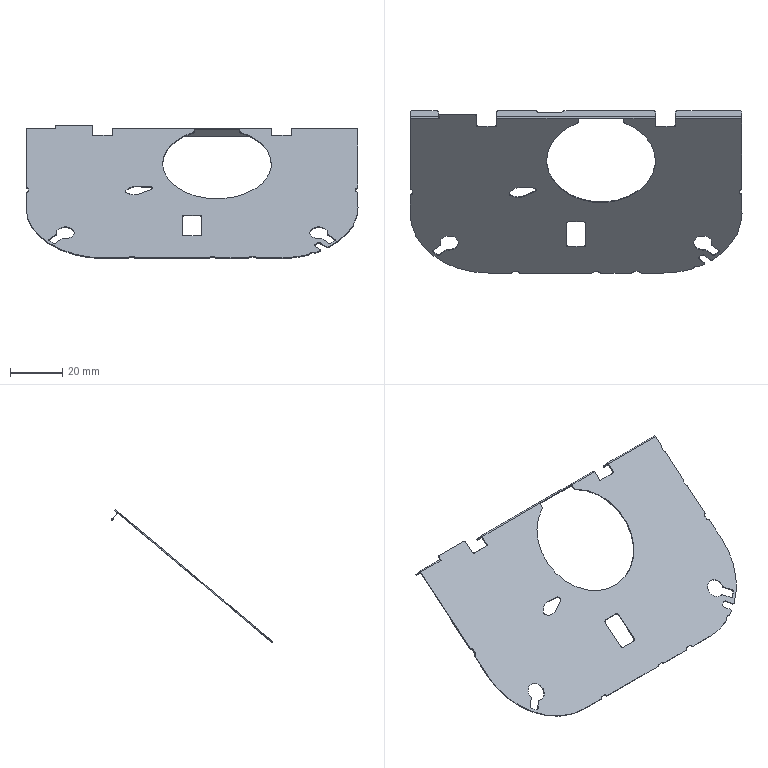Part | SolidWorks | features BaseBody 1 | 1 solid | 157 faces | box 127.4 x 62.108 x 51.15 mm | volume 3262 mm3 | cylinder 96 | plane 57 | spline 4 | commonest cylinder face diameters 1.3 x35 1 x15 7 x6 2 x5 0.6 x4 1.269 x4